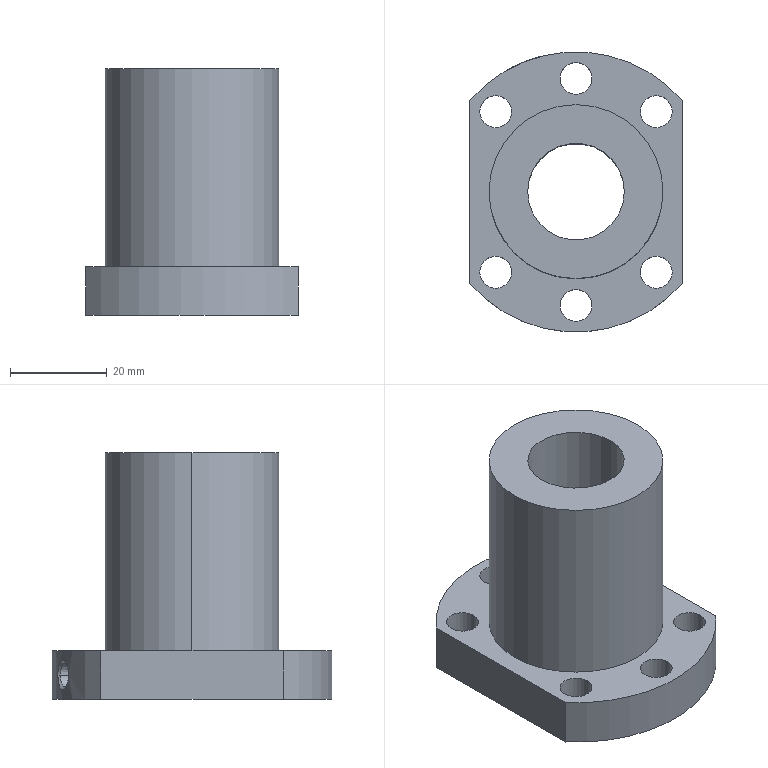Part | SolidWorks | features BaseBody 1 | 1 solid | 32 faces | box 44 x 58 x 51 mm | volume 46253 mm3 | cylinder 22 | plane 6 | cone 4 | commonest cylinder face diameters 6.6 x12 3 x2 4.917 x2 20 x2 36 x2 58 x2
STEP:
#1=CARTESIAN_POINT('',(-10.,0.,-61.));
#2=VERTEX_POINT('',#1);
#3=CARTESIAN_POINT('',(10.,0.,-61.));
#4=VERTEX_POINT('',#3);
#5=CARTESIAN_POINT('',(0.,0.,-61.));
#6=DIRECTION('',(0.,0.,1.));
#7=DIRECTION('',(1.,0.,0.));
#8=AXIS2_PLACEMENT_3D('',#5,#6,#7);
#9=CIRCLE('',#8,10.);
#10=EDGE_CURVE('',#2,#4,#9,.T.);
#11=ORIENTED_EDGE('',*,*,#10,.T.);
#12=CARTESIAN_POINT('',(10.,0.,-112.));
#13=VERTEX_POINT('',#12);
#14=CARTESIAN_POINT('',(10.,0.,-61.));
#15=DIRECTION('',(0.,0.,-1.));
#16=VECTOR('',#15,1000.);
#17=LINE('',#14,#16);
#18=EDGE_CURVE('',#4,#13,#17,.T.);
#19=ORIENTED_EDGE('',*,*,#18,.T.);
#20=CARTESIAN_POINT('',(-10.,0.,-112.));
#21=VERTEX_POINT('',#20);
#22=CARTESIAN_POINT('',(0.,0.,-112.));
#23=DIRECTION('',(0.,0.,1.));
#24=DIRECTION('',(1.,0.,0.));
#25=AXIS2_PLACEMENT_3D('',#22,#23,#24);
#26=CIRCLE('',#25,10.);
#27=EDGE_CURVE('',#21,#13,#26,.T.);
#28=ORIENTED_EDGE('',*,*,#27,.F.);
#29=CARTESIAN_POINT('',(-10.,0.,-61.));
#30=DIRECTION('',(0.,0.,-1.));
#31=VECTOR('',#30,1000.);
#32=LINE('',#29,#31);
#33=EDGE_CURVE('',#2,#21,#32,.T.);
#34=ORIENTED_EDGE('',*,*,#33,.F.);
#35=EDGE_LOOP('',(#11,#19,#28,#34));
#36=FACE_OUTER_BOUND('',#35,.T.);
#37=CARTESIAN_POINT('',(0.,0.,-61.));
#38=DIRECTION('',(0.,0.,-1.));
#39=DIRECTION('',(-1.,0.,0.));
#40=AXIS2_PLACEMENT_3D('',#37,#38,#39);
#41=CYLINDRICAL_SURFACE('',#40,10.);
#42=ADVANCED_FACE('',(#36),#41,.F.);
#43=CARTESIAN_POINT('',(-11.472,21.271,-107.));
#44=VERTEX_POINT('',#43);
#45=CARTESIAN_POINT('',(-6.929,23.152,-107.));
#46=VERTEX_POINT('',#45);
#47=CARTESIAN_POINT('',(-9.2,22.211,-107.));
#48=DIRECTION('',(0.3827,-0.9239,0.));
#49=DIRECTION('',(0.9239,0.3827,0.));
#50=AXIS2_PLACEMENT_3D('',#47,#48,#49);
#51=CIRCLE('',#50,2.459);
#52=EDGE_CURVE('',#44,#46,#51,.T.);
#53=ORIENTED_EDGE('',*,*,#52,.F.);
#54=CARTESIAN_POINT('',(-11.765,20.563,-107.));
#55=VERTEX_POINT('',#54);
#56=CARTESIAN_POINT('',(-11.472,21.271,-107.));
#57=DIRECTION('',(-0.3827,-0.9239,0.));
#58=VECTOR('',#57,1000.);
#59=LINE('',#56,#58);
#60=EDGE_CURVE('',#44,#55,#59,.T.);
#61=ORIENTED_EDGE('',*,*,#60,.T.);
#62=CARTESIAN_POINT('',(-6.221,22.859,-107.));
#63=VERTEX_POINT('',#62);
#64=CARTESIAN_POINT('',(-8.993,21.711,-107.));
#65=DIRECTION('',(0.3827,-0.9239,0.));
#66=DIRECTION('',(0.9239,0.3827,0.));
#67=AXIS2_PLACEMENT_3D('',#64,#65,#66);
#68=CIRCLE('',#67,3.);
#69=EDGE_CURVE('',#55,#63,#68,.T.);
#70=ORIENTED_EDGE('',*,*,#69,.T.);
#71=CARTESIAN_POINT('',(-6.929,23.152,-107.));
#72=DIRECTION('',(0.9239,-0.3827,0.));
#73=VECTOR('',#72,1000.);
#74=LINE('',#71,#73);
#75=EDGE_CURVE('',#46,#63,#74,.T.);
#76=ORIENTED_EDGE('',*,*,#75,.F.);
#77=EDGE_LOOP('',(#53,#61,#70,#76));
#78=FACE_OUTER_BOUND('',#77,.T.);
#79=CARTESIAN_POINT('',(-9.2,22.211,-107.));
#80=DIRECTION('',(0.3827,-0.9239,0.));
#81=DIRECTION('',(0.9239,0.3827,0.));
#82=AXIS2_PLACEMENT_3D('',#79,#80,#81);
#83=CONICAL_SURFACE('',#82,2.459,0.7854);
#84=ADVANCED_FACE('',(#78),#83,.F.);
#85=CARTESIAN_POINT('',(-13.162,25.351,-107.));
#86=VERTEX_POINT('',#85);
#87=CARTESIAN_POINT('',(-8.619,27.233,-107.));
#88=VERTEX_POINT('',#87);
#89=CARTESIAN_POINT('',(-10.891,26.292,-107.));
#90=DIRECTION('',(0.3827,-0.9239,0.));
#91=DIRECTION('',(0.9239,0.3827,0.));
#92=AXIS2_PLACEMENT_3D('',#89,#90,#91);
#93=CIRCLE('',#92,2.459);
#94=EDGE_CURVE('',#86,#88,#93,.T.);
#95=ORIENTED_EDGE('',*,*,#94,.F.);
#96=CARTESIAN_POINT('',(-5.279,6.319,-107.));
#97=DIRECTION('',(0.3827,-0.9239,0.));
#98=VECTOR('',#97,1000.);
#99=LINE('',#96,#98);
#100=EDGE_CURVE('',#86,#44,#99,.T.);
#101=ORIENTED_EDGE('',*,*,#100,.T.);
#102=ORIENTED_EDGE('',*,*,#52,.T.);
#103=CARTESIAN_POINT('',(-0.7358,8.201,-107.));
#104=DIRECTION('',(0.3827,-0.9239,0.));
#105=VECTOR('',#104,1000.);
#106=LINE('',#103,#105);
#107=EDGE_CURVE('',#88,#46,#106,.T.);
#108=ORIENTED_EDGE('',*,*,#107,.F.);
#109=EDGE_LOOP('',(#95,#101,#102,#108));
#110=FACE_OUTER_BOUND('',#109,.T.);
#111=CARTESIAN_POINT('',(-3.007,7.26,-107.));
#112=DIRECTION('',(0.3827,-0.9239,0.));
#113=DIRECTION('',(0.9239,0.3827,0.));
#114=AXIS2_PLACEMENT_3D('',#111,#112,#113);
#115=CYLINDRICAL_SURFACE('',#114,2.459);
#116=ADVANCED_FACE('',(#110),#115,.F.);
#117=ORIENTED_EDGE('',*,*,#94,.T.);
#118=CARTESIAN_POINT('',(-8.403,27.756,-107.));
#119=VERTEX_POINT('',#118);
#120=CARTESIAN_POINT('',(-8.326,27.941,-107.));
#121=DIRECTION('',(0.3827,0.9239,0.));
#122=VECTOR('',#121,1000.);
#123=LINE('',#120,#122);
#124=EDGE_CURVE('',#88,#119,#123,.T.);
#125=ORIENTED_EDGE('',*,*,#124,.T.);
#126=CARTESIAN_POINT('',(-13.685,25.568,-107.));
#127=VERTEX_POINT('',#126);
#128=CARTESIAN_POINT('',(-8.403,27.756,-107.));
#129=CARTESIAN_POINT('',(-8.403,27.756,-107.193));
#130=CARTESIAN_POINT('',(-8.42,27.751,-107.384));
#131=CARTESIAN_POINT('',(-8.486,27.731,-107.759));
#132=CARTESIAN_POINT('',(-8.537,27.715,-107.945));
#133=CARTESIAN_POINT('',(-8.67,27.674,-108.304));
#134=CARTESIAN_POINT('',(-8.751,27.648,-108.475));
#135=CARTESIAN_POINT('',(-8.943,27.587,-108.799));
#136=CARTESIAN_POINT('',(-9.056,27.55,-108.954));
#137=CARTESIAN_POINT('',(-9.304,27.467,-109.234));
#138=CARTESIAN_POINT('',(-9.439,27.421,-109.361));
#139=CARTESIAN_POINT('',(-9.732,27.319,-109.584));
#140=CARTESIAN_POINT('',(-9.891,27.262,-109.682));
#141=CARTESIAN_POINT('',(-10.219,27.141,-109.838));
#142=CARTESIAN_POINT('',(-10.388,27.076,-109.898));
#143=CARTESIAN_POINT('',(-10.739,26.939,-109.979));
#144=CARTESIAN_POINT('',(-10.917,26.867,-110.));
#145=CARTESIAN_POINT('',(-11.27,26.721,-110.));
#146=CARTESIAN_POINT('',(-11.448,26.645,-109.98));
#147=CARTESIAN_POINT('',(-11.793,26.495,-109.9));
#148=CARTESIAN_POINT('',(-11.959,26.42,-109.841));
#149=CARTESIAN_POINT('',(-12.277,26.274,-109.685));
#150=CARTESIAN_POINT('',(-12.43,26.201,-109.588));
#151=CARTESIAN_POINT('',(-12.71,26.067,-109.365));
#152=CARTESIAN_POINT('',(-12.84,26.003,-109.239));
#153=CARTESIAN_POINT('',(-13.076,25.885,-108.956));
#154=CARTESIAN_POINT('',(-13.18,25.832,-108.804));
#155=CARTESIAN_POINT('',(-13.36,25.739,-108.48));
#156=CARTESIAN_POINT('',(-13.437,25.699,-108.306));
#157=CARTESIAN_POINT('',(-13.56,25.634,-107.948));
#158=CARTESIAN_POINT('',(-13.607,25.61,-107.764));
#159=CARTESIAN_POINT('',(-13.669,25.577,-107.387));
#160=CARTESIAN_POINT('',(-13.685,25.568,-107.194));
#161=CARTESIAN_POINT('',(-13.685,25.568,-107.));
#162=B_SPLINE_CURVE_WITH_KNOTS('',3,(#128,#129,#130,#131,#132,#133,#134,#135,#136,#137,#138,#139,#140,#141,#142,#143,#144,#145,#146,#147,#148,#149,#150,#151,#152,#153,#154,#155,#156,#157,#158,#159,#160,#161),.UNSPECIFIED.,.F.,.F.,(4,2,2,2,2,2,2,2,2,2,2,2,2,2,2,2,4),(0.000000001,0.0005722,0.001144,0.001717,0.002289,0.002861,0.003433,0.004006,0.004578,0.00515,0.005722,0.006295,0.006867,0.007439,0.008011,0.008584,0.009156),.UNSPECIFIED.);
#163=EDGE_CURVE('',#119,#127,#162,.T.);
#164=ORIENTED_EDGE('',*,*,#163,.T.);
#165=CARTESIAN_POINT('',(-13.869,25.644,-107.));
#166=DIRECTION('',(-0.9239,0.3827,0.));
#167=VECTOR('',#166,1000.);
#168=LINE('',#165,#167);
#169=EDGE_CURVE('',#86,#127,#168,.T.);
#170=ORIENTED_EDGE('',*,*,#169,.F.);
#171=EDGE_LOOP('',(#117,#125,#164,#170));
#172=FACE_OUTER_BOUND('',#171,.T.);
#173=CARTESIAN_POINT('',(-11.098,26.793,-107.));
#174=DIRECTION('',(-0.3827,0.9239,0.));
#175=DIRECTION('',(-0.9239,-0.3827,0.));
#176=AXIS2_PLACEMENT_3D('',#173,#174,#175);
#177=CONICAL_SURFACE('',#176,3.,0.7854);
#178=ADVANCED_FACE('',(#172),#177,.F.);
#179=CARTESIAN_POINT('',(-19.917,16.617,-102.));
#180=VERTEX_POINT('',#179);
#181=CARTESIAN_POINT('',(-13.317,16.617,-102.));
#182=VERTEX_POINT('',#181);
#183=CARTESIAN_POINT('',(-16.617,16.617,-102.));
#184=DIRECTION('',(0.,0.,1.));
#185=DIRECTION('',(1.,0.,0.));
#186=AXIS2_PLACEMENT_3D('',#183,#184,#185);
#187=CIRCLE('',#186,3.3);
#188=EDGE_CURVE('',#180,#182,#187,.T.);
#189=ORIENTED_EDGE('',*,*,#188,.T.);
#190=CARTESIAN_POINT('',(-13.317,16.617,-112.));
#191=VERTEX_POINT('',#190);
#192=CARTESIAN_POINT('',(-13.317,16.617,-102.));
#193=DIRECTION('',(0.,0.,-1.));
#194=VECTOR('',#193,1000.);
#195=LINE('',#192,#194);
#196=EDGE_CURVE('',#182,#191,#195,.T.);
#197=ORIENTED_EDGE('',*,*,#196,.T.);
#198=CARTESIAN_POINT('',(-19.917,16.617,-112.));
#199=VERTEX_POINT('',#198);
#200=CARTESIAN_POINT('',(-16.617,16.617,-112.));
#201=DIRECTION('',(0.,0.,1.));
#202=DIRECTION('',(1.,0.,0.));
#203=AXIS2_PLACEMENT_3D('',#200,#201,#202);
#204=CIRCLE('',#203,3.3);
#205=EDGE_CURVE('',#199,#191,#204,.T.);
#206=ORIENTED_EDGE('',*,*,#205,.F.);
#207=CARTESIAN_POINT('',(-19.917,16.617,-102.));
#208=DIRECTION('',(0.,0.,-1.));
#209=VECTOR('',#208,1000.);
#210=LINE('',#207,#209);
#211=EDGE_CURVE('',#180,#199,#210,.T.);
#212=ORIENTED_EDGE('',*,*,#211,.F.);
#213=EDGE_LOOP('',(#189,#197,#206,#212));
#214=FACE_OUTER_BOUND('',#213,.T.);
#215=CARTESIAN_POINT('',(-16.617,16.617,-102.));
#216=DIRECTION('',(0.,0.,-1.));
#217=DIRECTION('',(-1.,0.,0.));
#218=AXIS2_PLACEMENT_3D('',#215,#216,#217);
#219=CYLINDRICAL_SURFACE('',#218,3.3);
#220=ADVANCED_FACE('',(#214),#219,.F.);
#221=CARTESIAN_POINT('',(-19.917,-16.617,-102.));
#222=VERTEX_POINT('',#221);
#223=CARTESIAN_POINT('',(-13.317,-16.617,-102.));
#224=VERTEX_POINT('',#223);
#225=CARTESIAN_POINT('',(-16.617,-16.617,-102.));
#226=DIRECTION('',(0.,0.,1.));
#227=DIRECTION('',(1.,0.,0.));
#228=AXIS2_PLACEMENT_3D('',#225,#226,#227);
#229=CIRCLE('',#228,3.3);
#230=EDGE_CURVE('',#222,#224,#229,.T.);
#231=ORIENTED_EDGE('',*,*,#230,.T.);
#232=CARTESIAN_POINT('',(-13.317,-16.617,-112.));
#233=VERTEX_POINT('',#232);
#234=CARTESIAN_POINT('',(-13.317,-16.617,-102.));
#235=DIRECTION('',(0.,0.,-1.));
#236=VECTOR('',#235,1000.);
#237=LINE('',#234,#236);
#238=EDGE_CURVE('',#224,#233,#237,.T.);
#239=ORIENTED_EDGE('',*,*,#238,.T.);
#240=CARTESIAN_POINT('',(-19.917,-16.617,-112.));
#241=VERTEX_POINT('',#240);
#242=CARTESIAN_POINT('',(-16.617,-16.617,-112.));
#243=DIRECTION('',(0.,0.,1.));
#244=DIRECTION('',(1.,0.,0.));
#245=AXIS2_PLACEMENT_3D('',#242,#243,#244);
#246=CIRCLE('',#245,3.3);
#247=EDGE_CURVE('',#241,#233,#246,.T.);
#248=ORIENTED_EDGE('',*,*,#247,.F.);
#249=CARTESIAN_POINT('',(-19.917,-16.617,-102.));
#250=DIRECTION('',(0.,0.,-1.));
#251=VECTOR('',#250,1000.);
#252=LINE('',#249,#251);
#253=EDGE_CURVE('',#222,#241,#252,.T.);
#254=ORIENTED_EDGE('',*,*,#253,.F.);
#255=EDGE_LOOP('',(#231,#239,#248,#254));
#256=FACE_OUTER_BOUND('',#255,.T.);
#257=CARTESIAN_POINT('',(-16.617,-16.617,-102.));
#258=DIRECTION('',(0.,0.,-1.));
#259=DIRECTION('',(-1.,0.,0.));
#260=AXIS2_PLACEMENT_3D('',#257,#258,#259);
#261=CYLINDRICAL_SURFACE('',#260,3.3);
#262=ADVANCED_FACE('',(#256),#261,.F.);
#263=CARTESIAN_POINT('',(-3.3,-23.5,-102.));
#264=VERTEX_POINT('',#263);
#265=CARTESIAN_POINT('',(3.3,-23.5,-102.));
#266=VERTEX_POINT('',#265);
#267=CARTESIAN_POINT('',(0.,-23.5,-102.));
#268=DIRECTION('',(0.,0.,1.));
#269=DIRECTION('',(1.,0.,0.));
#270=AXIS2_PLACEMENT_3D('',#267,#268,#269);
#271=CIRCLE('',#270,3.3);
#272=EDGE_CURVE('',#264,#266,#271,.T.);
#273=ORIENTED_EDGE('',*,*,#272,.T.);
#274=CARTESIAN_POINT('',(3.3,-23.5,-112.));
#275=VERTEX_POINT('',#274);
#276=CARTESIAN_POINT('',(3.3,-23.5,-102.));
#277=DIRECTION('',(0.,0.,-1.));
#278=VECTOR('',#277,1000.);
#279=LINE('',#276,#278);
#280=EDGE_CURVE('',#266,#275,#279,.T.);
#281=ORIENTED_EDGE('',*,*,#280,.T.);
#282=CARTESIAN_POINT('',(-3.3,-23.5,-112.));
#283=VERTEX_POINT('',#282);
#284=CARTESIAN_POINT('',(0.,-23.5,-112.));
#285=DIRECTION('',(0.,0.,1.));
#286=DIRECTION('',(1.,0.,0.));
#287=AXIS2_PLACEMENT_3D('',#284,#285,#286);
#288=CIRCLE('',#287,3.3);
#289=EDGE_CURVE('',#283,#275,#288,.T.);
#290=ORIENTED_EDGE('',*,*,#289,.F.);
#291=CARTESIAN_POINT('',(-3.3,-23.5,-102.));
#292=DIRECTION('',(0.,0.,-1.));
#293=VECTOR('',#292,1000.);
#294=LINE('',#291,#293);
#295=EDGE_CURVE('',#264,#283,#294,.T.);
#296=ORIENTED_EDGE('',*,*,#295,.F.);
#297=EDGE_LOOP('',(#273,#281,#290,#296));
#298=FACE_OUTER_BOUND('',#297,.T.);
#299=CARTESIAN_POINT('',(0.,-23.5,-102.));
#300=DIRECTION('',(0.,0.,-1.));
#301=DIRECTION('',(-1.,0.,0.));
#302=AXIS2_PLACEMENT_3D('',#299,#300,#301);
#303=CYLINDRICAL_SURFACE('',#302,3.3);
#304=ADVANCED_FACE('',(#298),#303,.F.);
#305=CARTESIAN_POINT('',(-3.3,23.5,-102.));
#306=VERTEX_POINT('',#305);
#307=CARTESIAN_POINT('',(3.3,23.5,-102.));
#308=VERTEX_POINT('',#307);
#309=CARTESIAN_POINT('',(0.,23.5,-102.));
#310=DIRECTION('',(0.,0.,1.));
#311=DIRECTION('',(1.,0.,0.));
#312=AXIS2_PLACEMENT_3D('',#309,#310,#311);
#313=CIRCLE('',#312,3.3);
#314=EDGE_CURVE('',#306,#308,#313,.T.);
#315=ORIENTED_EDGE('',*,*,#314,.T.);
#316=CARTESIAN_POINT('',(3.3,23.5,-112.));
#317=VERTEX_POINT('',#316);
#318=CARTESIAN_POINT('',(3.3,23.5,-102.));
#319=DIRECTION('',(0.,0.,-1.));
#320=VECTOR('',#319,1000.);
#321=LINE('',#318,#320);
#322=EDGE_CURVE('',#308,#317,#321,.T.);
#323=ORIENTED_EDGE('',*,*,#322,.T.);
#324=CARTESIAN_POINT('',(-3.3,23.5,-112.));
#325=VERTEX_POINT('',#324);
#326=CARTESIAN_POINT('',(0.,23.5,-112.));
#327=DIRECTION('',(0.,0.,1.));
#328=DIRECTION('',(1.,0.,0.));
#329=AXIS2_PLACEMENT_3D('',#326,#327,#328);
#330=CIRCLE('',#329,3.3);
#331=EDGE_CURVE('',#325,#317,#330,.T.);
#332=ORIENTED_EDGE('',*,*,#331,.F.);
#333=CARTESIAN_POINT('',(-3.3,23.5,-102.));
#334=DIRECTION('',(0.,0.,-1.));
#335=VECTOR('',#334,1000.);
#336=LINE('',#333,#335);
#337=EDGE_CURVE('',#306,#325,#336,.T.);
#338=ORIENTED_EDGE('',*,*,#337,.F.);
#339=EDGE_LOOP('',(#315,#323,#332,#338));
#340=FACE_OUTER_BOUND('',#339,.T.);
#341=CARTESIAN_POINT('',(0.,23.5,-102.));
#342=DIRECTION('',(0.,0.,-1.));
#343=DIRECTION('',(-1.,0.,0.));
#344=AXIS2_PLACEMENT_3D('',#341,#342,#343);
#345=CYLINDRICAL_SURFACE('',#344,3.3);
#346=ADVANCED_FACE('',(#340),#345,.F.);
#347=CARTESIAN_POINT('',(13.317,-16.617,-102.));
#348=VERTEX_POINT('',#347);
#349=CARTESIAN_POINT('',(19.917,-16.617,-102.));
#350=VERTEX_POINT('',#349);
#351=CARTESIAN_POINT('',(16.617,-16.617,-102.));
#352=DIRECTION('',(0.,0.,1.));
#353=DIRECTION('',(1.,0.,0.));
#354=AXIS2_PLACEMENT_3D('',#351,#352,#353);
#355=CIRCLE('',#354,3.3);
#356=EDGE_CURVE('',#348,#350,#355,.T.);
#357=ORIENTED_EDGE('',*,*,#356,.T.);
#358=CARTESIAN_POINT('',(19.917,-16.617,-112.));
#359=VERTEX_POINT('',#358);
#360=CARTESIAN_POINT('',(19.917,-16.617,-102.));
#361=DIRECTION('',(0.,0.,-1.));
#362=VECTOR('',#361,1000.);
#363=LINE('',#360,#362);
#364=EDGE_CURVE('',#350,#359,#363,.T.);
#365=ORIENTED_EDGE('',*,*,#364,.T.);
#366=CARTESIAN_POINT('',(13.317,-16.617,-112.));
#367=VERTEX_POINT('',#366);
#368=CARTESIAN_POINT('',(16.617,-16.617,-112.));
#369=DIRECTION('',(0.,0.,1.));
#370=DIRECTION('',(1.,0.,0.));
#371=AXIS2_PLACEMENT_3D('',#368,#369,#370);
#372=CIRCLE('',#371,3.3);
#373=EDGE_CURVE('',#367,#359,#372,.T.);
#374=ORIENTED_EDGE('',*,*,#373,.F.);
#375=CARTESIAN_POINT('',(13.317,-16.617,-102.));
#376=DIRECTION('',(0.,0.,-1.));
#377=VECTOR('',#376,1000.);
#378=LINE('',#375,#377);
#379=EDGE_CURVE('',#348,#367,#378,.T.);
#380=ORIENTED_EDGE('',*,*,#379,.F.);
#381=EDGE_LOOP('',(#357,#365,#374,#380));
#382=FACE_OUTER_BOUND('',#381,.T.);
#383=CARTESIAN_POINT('',(16.617,-16.617,-102.));
#384=DIRECTION('',(0.,0.,-1.));
#385=DIRECTION('',(-1.,0.,0.));
#386=AXIS2_PLACEMENT_3D('',#383,#384,#385);
#387=CYLINDRICAL_SURFACE('',#386,3.3);
#388=ADVANCED_FACE('',(#382),#387,.F.);
#389=CARTESIAN_POINT('',(13.317,16.617,-102.));
#390=VERTEX_POINT('',#389);
#391=CARTESIAN_POINT('',(19.917,16.617,-102.));
#392=VERTEX_POINT('',#391);
#393=CARTESIAN_POINT('',(16.617,16.617,-102.));
#394=DIRECTION('',(0.,0.,1.));
#395=DIRECTION('',(1.,0.,0.));
#396=AXIS2_PLACEMENT_3D('',#393,#394,#395);
#397=CIRCLE('',#396,3.3);
#398=EDGE_CURVE('',#390,#392,#397,.T.);
#399=ORIENTED_EDGE('',*,*,#398,.T.);
#400=CARTESIAN_POINT('',(19.917,16.617,-112.));
#401=VERTEX_POINT('',#400);
#402=CARTESIAN_POINT('',(19.917,16.617,-102.));
#403=DIRECTION('',(0.,0.,-1.));
#404=VECTOR('',#403,1000.);
#405=LINE('',#402,#404);
#406=EDGE_CURVE('',#392,#401,#405,.T.);
#407=ORIENTED_EDGE('',*,*,#406,.T.);
#408=CARTESIAN_POINT('',(13.317,16.617,-112.));
#409=VERTEX_POINT('',#408);
#410=CARTESIAN_POINT('',(16.617,16.617,-112.));
#411=DIRECTION('',(0.,0.,1.));
#412=DIRECTION('',(1.,0.,0.));
#413=AXIS2_PLACEMENT_3D('',#410,#411,#412);
#414=CIRCLE('',#413,3.3);
#415=EDGE_CURVE('',#409,#401,#414,.T.);
#416=ORIENTED_EDGE('',*,*,#415,.F.);
#417=CARTESIAN_POINT('',(13.317,16.617,-102.));
#418=DIRECTION('',(0.,0.,-1.));
#419=VECTOR('',#418,1000.);
#420=LINE('',#417,#419);
#421=EDGE_CURVE('',#390,#409,#420,.T.);
#422=ORIENTED_EDGE('',*,*,#421,.F.);
#423=EDGE_LOOP('',(#399,#407,#416,#422));
#424=FACE_OUTER_BOUND('',#423,.T.);
#425=CARTESIAN_POINT('',(16.617,16.617,-102.));
#426=DIRECTION('',(0.,0.,-1.));
#427=DIRECTION('',(-1.,0.,0.));
#428=AXIS2_PLACEMENT_3D('',#425,#426,#427);
#429=CYLINDRICAL_SURFACE('',#428,3.3);
#430=ADVANCED_FACE('',(#424),#429,.F.);
#431=CARTESIAN_POINT('',(18.,0.,-61.));
#432=VERTEX_POINT('',#431);
#433=CARTESIAN_POINT('',(-18.,0.,-61.));
#434=VERTEX_POINT('',#433);
#435=CARTESIAN_POINT('',(0.,0.,-61.));
#436=DIRECTION('',(0.,0.,1.));
#437=DIRECTION('',(1.,0.,0.));
#438=AXIS2_PLACEMENT_3D('',#435,#436,#437);
#439=CIRCLE('',#438,18.);
#440=EDGE_CURVE('',#432,#434,#439,.T.);
#441=ORIENTED_EDGE('',*,*,#440,.F.);
#442=CARTESIAN_POINT('',(18.,0.,-102.));
#443=VERTEX_POINT('',#442);
#444=CARTESIAN_POINT('',(18.,0.,-61.));
#445=DIRECTION('',(0.,0.,-1.));
#446=VECTOR('',#445,1000.);
#447=LINE('',#444,#446);
#448=EDGE_CURVE('',#432,#443,#447,.T.);
#449=ORIENTED_EDGE('',*,*,#448,.T.);
#450=CARTESIAN_POINT('',(-18.,0.,-102.));
#451=VERTEX_POINT('',#450);
#452=CARTESIAN_POINT('',(0.,0.,-102.));
#453=DIRECTION('',(0.,0.,1.));
#454=DIRECTION('',(1.,0.,0.));
#455=AXIS2_PLACEMENT_3D('',#452,#453,#454);
#456=CIRCLE('',#455,18.);
#457=EDGE_CURVE('',#443,#451,#456,.T.);
#458=ORIENTED_EDGE('',*,*,#457,.T.);
#459=CARTESIAN_POINT('',(-18.,0.,-61.));
#460=DIRECTION('',(0.,0.,-1.));
#461=VECTOR('',#460,1000.);
#462=LINE('',#459,#461);
#463=EDGE_CURVE('',#434,#451,#462,.T.);
#464=ORIENTED_EDGE('',*,*,#463,.F.);
#465=EDGE_LOOP('',(#441,#449,#458,#464));
#466=FACE_OUTER_BOUND('',#465,.T.);
#467=CARTESIAN_POINT('',(0.,0.,-61.));
#468=DIRECTION('',(0.,0.,-1.));
#469=DIRECTION('',(-1.,0.,0.));
#470=AXIS2_PLACEMENT_3D('',#467,#468,#469);
#471=CYLINDRICAL_SURFACE('',#470,18.);
#472=ADVANCED_FACE('',(#466),#471,.T.);
#473=CARTESIAN_POINT('',(-10.379,21.137,-107.));
#474=VERTEX_POINT('',#473);
#475=CARTESIAN_POINT('',(-7.607,22.285,-107.));
#476=VERTEX_POINT('',#475);
#477=CARTESIAN_POINT('',(-8.993,21.711,-107.));
#478=DIRECTION('',(0.3827,-0.9239,0.));
#479=DIRECTION('',(0.9239,0.3827,0.));
#480=AXIS2_PLACEMENT_3D('',#477,#478,#479);
#481=CIRCLE('',#480,1.5);
#482=EDGE_CURVE('',#474,#476,#481,.T.);
#483=ORIENTED_EDGE('',*,*,#482,.F.);
#484=CARTESIAN_POINT('',(-5.169,8.56,-107.));
#485=VERTEX_POINT('',#484);
#486=CARTESIAN_POINT('',(-4.393,6.686,-107.));
#487=DIRECTION('',(0.3827,-0.9239,0.));
#488=VECTOR('',#487,1000.);
#489=LINE('',#486,#488);
#490=EDGE_CURVE('',#474,#485,#489,.T.);
#491=ORIENTED_EDGE('',*,*,#490,.T.);
#492=CARTESIAN_POINT('',(-2.398,9.708,-107.));
#493=VERTEX_POINT('',#492);
#494=CARTESIAN_POINT('',(-5.169,8.56,-107.));
#495=CARTESIAN_POINT('',(-5.169,8.56,-107.099));
#496=CARTESIAN_POINT('',(-5.161,8.565,-107.197));
#497=CARTESIAN_POINT('',(-5.128,8.585,-107.389));
#498=CARTESIAN_POINT('',(-5.103,8.6,-107.484));
#499=CARTESIAN_POINT('',(-5.037,8.639,-107.666));
#500=CARTESIAN_POINT('',(-4.997,8.662,-107.752));
#501=CARTESIAN_POINT('',(-4.902,8.716,-107.915));
#502=CARTESIAN_POINT('',(-4.846,8.748,-107.992));
#503=CARTESIAN_POINT('',(-4.663,8.847,-108.199));
#504=CARTESIAN_POINT('',(-4.514,8.925,-108.311));
#505=CARTESIAN_POINT('',(-4.189,9.082,-108.46));
#506=CARTESIAN_POINT('',(-4.009,9.163,-108.5));
#507=CARTESIAN_POINT('',(-3.737,9.276,-108.5));
#508=CARTESIAN_POINT('',(-3.645,9.313,-108.49));
#509=CARTESIAN_POINT('',(-3.465,9.381,-108.452));
#510=CARTESIAN_POINT('',(-3.377,9.413,-108.424));
#511=CARTESIAN_POINT('',(-3.119,9.503,-108.311));
#512=CARTESIAN_POINT('',(-2.961,9.553,-108.201));
#513=CARTESIAN_POINT('',(-2.758,9.612,-107.991));
#514=CARTESIAN_POINT('',(-2.698,9.629,-107.916));
#515=CARTESIAN_POINT('',(-2.593,9.658,-107.754));
#516=CARTESIAN_POINT('',(-2.547,9.67,-107.666));
#517=CARTESIAN_POINT('',(-2.436,9.699,-107.394));
#518=CARTESIAN_POINT('',(-2.398,9.708,-107.198));
#519=CARTESIAN_POINT('',(-2.398,9.708,-107.));
#520=B_SPLINE_CURVE_WITH_KNOTS('',3,(#494,#495,#496,#497,#498,#499,#500,#501,#502,#503,#504,#505,#506,#507,#508,#509,#510,#511,#512,#513,#514,#515,#516,#517,#518,#519),.UNSPECIFIED.,.F.,.F.,(4,2,2,2,2,2,2,2,2,2,2,2,4),(0.,0.0002934,0.0005869,0.0008803,0.001174,0.001761,0.002348,0.002641,0.002934,0.003521,0.003815,0.004108,0.004695),.UNSPECIFIED.);
#521=EDGE_CURVE('',#485,#493,#520,.T.);
#522=ORIENTED_EDGE('',*,*,#521,.T.);
#523=CARTESIAN_POINT('',(-1.621,7.834,-107.));
#524=DIRECTION('',(0.3827,-0.9239,0.));
#525=VECTOR('',#524,1000.);
#526=LINE('',#523,#525);
#527=EDGE_CURVE('',#476,#493,#526,.T.);
#528=ORIENTED_EDGE('',*,*,#527,.F.);
#529=EDGE_LOOP('',(#483,#491,#522,#528));
#530=FACE_OUTER_BOUND('',#529,.T.);
#531=CARTESIAN_POINT('',(-3.007,7.26,-107.));
#532=DIRECTION('',(0.3827,-0.9239,0.));
#533=DIRECTION('',(0.9239,0.3827,0.));
#534=AXIS2_PLACEMENT_3D('',#531,#532,#533);
#535=CYLINDRICAL_SURFACE('',#534,1.5);
#536=ADVANCED_FACE('',(#530),#535,.F.);
#537=CARTESIAN_POINT('',(-8.993,21.711,-107.));
#538=DIRECTION('',(0.3827,-0.9239,0.));
#539=DIRECTION('',(0.9239,0.3827,0.));
#540=AXIS2_PLACEMENT_3D('',#537,#538,#539);
#541=CIRCLE('',#540,1.5);
#542=EDGE_CURVE('',#476,#474,#541,.T.);
#543=ORIENTED_EDGE('',*,*,#542,.T.);
#544=ORIENTED_EDGE('',*,*,#482,.T.);
#545=EDGE_LOOP('',(#543,#544));
#546=FACE_BOUND('',#545,.T.);
#547=CARTESIAN_POINT('',(-8.993,21.711,-107.));
#548=DIRECTION('',(0.3827,-0.9239,0.));
#549=DIRECTION('',(0.9239,0.3827,0.));
#550=AXIS2_PLACEMENT_3D('',#547,#548,#549);
#551=CIRCLE('',#550,3.);
#552=EDGE_CURVE('',#63,#55,#551,.T.);
#553=ORIENTED_EDGE('',*,*,#552,.F.);
#554=ORIENTED_EDGE('',*,*,#69,.F.);
#555=EDGE_LOOP('',(#553,#554));
#556=FACE_OUTER_BOUND('',#555,.T.);
#557=CARTESIAN_POINT('',(-6.221,22.859,-107.));
#558=DIRECTION('',(-0.3827,0.9239,0.));
#559=DIRECTION('',(0.,0.,1.));
#560=AXIS2_PLACEMENT_3D('',#557,#558,#559);
#561=PLANE('',#560);
#562=ADVANCED_FACE('',(#546,#556),#561,.T.);
#563=ORIENTED_EDGE('',*,*,#415,.T.);
#564=CARTESIAN_POINT('',(16.617,16.617,-112.));
#565=DIRECTION('',(0.,0.,1.));
#566=DIRECTION('',(1.,0.,0.));
#567=AXIS2_PLACEMENT_3D('',#564,#565,#566);
#568=CIRCLE('',#567,3.3);
#569=EDGE_CURVE('',#401,#409,#568,.T.);
#570=ORIENTED_EDGE('',*,*,#569,.T.);
#571=EDGE_LOOP('',(#563,#570));
#572=FACE_BOUND('',#571,.T.);
#573=ORIENTED_EDGE('',*,*,#373,.T.);
#574=CARTESIAN_POINT('',(16.617,-16.617,-112.));
#575=DIRECTION('',(0.,0.,1.));
#576=DIRECTION('',(1.,0.,0.));
#577=AXIS2_PLACEMENT_3D('',#574,#575,#576);
#578=CIRCLE('',#577,3.3);
#579=EDGE_CURVE('',#359,#367,#578,.T.);
#580=ORIENTED_EDGE('',*,*,#579,.T.);
#581=EDGE_LOOP('',(#573,#580));
#582=FACE_BOUND('',#581,.T.);
#583=ORIENTED_EDGE('',*,*,#331,.T.);
#584=CARTESIAN_POINT('',(0.,23.5,-112.));
#585=DIRECTION('',(0.,0.,1.));
#586=DIRECTION('',(1.,0.,0.));
#587=AXIS2_PLACEMENT_3D('',#584,#585,#586);
#588=CIRCLE('',#587,3.3);
#589=EDGE_CURVE('',#317,#325,#588,.T.);
#590=ORIENTED_EDGE('',*,*,#589,.T.);
#591=EDGE_LOOP('',(#583,#590));
#592=FACE_BOUND('',#591,.T.);
#593=ORIENTED_EDGE('',*,*,#289,.T.);
#594=CARTESIAN_POINT('',(0.,-23.5,-112.));
#595=DIRECTION('',(0.,0.,1.));
#596=DIRECTION('',(1.,0.,0.));
#597=AXIS2_PLACEMENT_3D('',#594,#595,#596);
#598=CIRCLE('',#597,3.3);
#599=EDGE_CURVE('',#275,#283,#598,.T.);
#600=ORIENTED_EDGE('',*,*,#599,.T.);
#601=EDGE_LOOP('',(#593,#600));
#602=FACE_BOUND('',#601,.T.);
#603=ORIENTED_EDGE('',*,*,#247,.T.);
#604=CARTESIAN_POINT('',(-16.617,-16.617,-112.));
#605=DIRECTION('',(0.,0.,1.));
#606=DIRECTION('',(1.,0.,0.));
#607=AXIS2_PLACEMENT_3D('',#604,#605,#606);
#608=CIRCLE('',#607,3.3);
#609=EDGE_CURVE('',#233,#241,#608,.T.);
#610=ORIENTED_EDGE('',*,*,#609,.T.);
#611=EDGE_LOOP('',(#603,#610));
#612=FACE_BOUND('',#611,.T.);
#613=ORIENTED_EDGE('',*,*,#205,.T.);
#614=CARTESIAN_POINT('',(-16.617,16.617,-112.));
#615=DIRECTION('',(0.,0.,1.));
#616=DIRECTION('',(1.,0.,0.));
#617=AXIS2_PLACEMENT_3D('',#614,#615,#616);
#618=CIRCLE('',#617,3.3);
#619=EDGE_CURVE('',#191,#199,#618,.T.);
#620=ORIENTED_EDGE('',*,*,#619,.T.);
#621=EDGE_LOOP('',(#613,#620));
#622=FACE_BOUND('',#621,.T.);
#623=ORIENTED_EDGE('',*,*,#27,.T.);
#624=CARTESIAN_POINT('',(0.,0.,-112.));
#625=DIRECTION('',(0.,0.,1.));
#626=DIRECTION('',(1.,0.,0.));
#627=AXIS2_PLACEMENT_3D('',#624,#625,#626);
#628=CIRCLE('',#627,10.);
#629=EDGE_CURVE('',#13,#21,#628,.T.);
#630=ORIENTED_EDGE('',*,*,#629,.T.);
#631=EDGE_LOOP('',(#623,#630));
#632=FACE_BOUND('',#631,.T.);
#633=CARTESIAN_POINT('',(22.,18.894,-112.));
#634=VERTEX_POINT('',#633);
#635=CARTESIAN_POINT('',(-22.,18.894,-112.));
#636=VERTEX_POINT('',#635);
#637=CARTESIAN_POINT('',(0.,0.,-112.));
#638=DIRECTION('',(0.,0.,1.));
#639=DIRECTION('',(1.,0.,0.));
#640=AXIS2_PLACEMENT_3D('',#637,#638,#639);
#641=CIRCLE('',#640,29.);
#642=EDGE_CURVE('',#634,#636,#641,.T.);
#643=ORIENTED_EDGE('',*,*,#642,.F.);
#644=CARTESIAN_POINT('',(22.,-18.894,-112.));
#645=VERTEX_POINT('',#644);
#646=CARTESIAN_POINT('',(22.,-18.894,-112.));
#647=DIRECTION('',(0.,1.,0.));
#648=VECTOR('',#647,1000.);
#649=LINE('',#646,#648);
#650=EDGE_CURVE('',#645,#634,#649,.T.);
#651=ORIENTED_EDGE('',*,*,#650,.F.);
#652=CARTESIAN_POINT('',(-22.,-18.894,-112.));
#653=VERTEX_POINT('',#652);
#654=CARTESIAN_POINT('',(0.,0.,-112.));
#655=DIRECTION('',(0.,0.,1.));
#656=DIRECTION('',(1.,0.,0.));
#657=AXIS2_PLACEMENT_3D('',#654,#655,#656);
#658=CIRCLE('',#657,29.);
#659=EDGE_CURVE('',#653,#645,#658,.T.);
#660=ORIENTED_EDGE('',*,*,#659,.F.);
#661=CARTESIAN_POINT('',(-22.,18.894,-112.));
#662=DIRECTION('',(0.,-1.,0.));
#663=VECTOR('',#662,1000.);
#664=LINE('',#661,#663);
#665=EDGE_CURVE('',#636,#653,#664,.T.);
#666=ORIENTED_EDGE('',*,*,#665,.F.);
#667=EDGE_LOOP('',(#643,#651,#660,#666));
#668=FACE_OUTER_BOUND('',#667,.T.);
#669=CARTESIAN_POINT('',(0.,0.,-112.));
#670=DIRECTION('',(0.,0.,1.));
#671=DIRECTION('',(1.,0.,0.));
#672=AXIS2_PLACEMENT_3D('',#669,#670,#671);
#673=PLANE('',#672);
#674=ADVANCED_FACE('',(#572,#582,#592,#602,#612,#622,#632,#668),#673,.F.);
#675=ORIENTED_EDGE('',*,*,#398,.F.);
#676=CARTESIAN_POINT('',(16.617,16.617,-102.));
#677=DIRECTION('',(0.,0.,1.));
#678=DIRECTION('',(1.,0.,0.));
#679=AXIS2_PLACEMENT_3D('',#676,#677,#678);
#680=CIRCLE('',#679,3.3);
#681=EDGE_CURVE('',#392,#390,#680,.T.);
#682=ORIENTED_EDGE('',*,*,#681,.F.);
#683=EDGE_LOOP('',(#675,#682));
#684=FACE_BOUND('',#683,.T.);
#685=ORIENTED_EDGE('',*,*,#356,.F.);
#686=CARTESIAN_POINT('',(16.617,-16.617,-102.));
#687=DIRECTION('',(0.,0.,1.));
#688=DIRECTION('',(1.,0.,0.));
#689=AXIS2_PLACEMENT_3D('',#686,#687,#688);
#690=CIRCLE('',#689,3.3);
#691=EDGE_CURVE('',#350,#348,#690,.T.);
#692=ORIENTED_EDGE('',*,*,#691,.F.);
#693=EDGE_LOOP('',(#685,#692));
#694=FACE_BOUND('',#693,.T.);
#695=ORIENTED_EDGE('',*,*,#314,.F.);
#696=CARTESIAN_POINT('',(0.,23.5,-102.));
#697=DIRECTION('',(0.,0.,1.));
#698=DIRECTION('',(1.,0.,0.));
#699=AXIS2_PLACEMENT_3D('',#696,#697,#698);
#700=CIRCLE('',#699,3.3);
#701=EDGE_CURVE('',#308,#306,#700,.T.);
#702=ORIENTED_EDGE('',*,*,#701,.F.);
#703=EDGE_LOOP('',(#695,#702));
#704=FACE_BOUND('',#703,.T.);
#705=ORIENTED_EDGE('',*,*,#272,.F.);
#706=CARTESIAN_POINT('',(0.,-23.5,-102.));
#707=DIRECTION('',(0.,0.,1.));
#708=DIRECTION('',(1.,0.,0.));
#709=AXIS2_PLACEMENT_3D('',#706,#707,#708);
#710=CIRCLE('',#709,3.3);
#711=EDGE_CURVE('',#266,#264,#710,.T.);
#712=ORIENTED_EDGE('',*,*,#711,.F.);
#713=EDGE_LOOP('',(#705,#712));
#714=FACE_BOUND('',#713,.T.);
#715=ORIENTED_EDGE('',*,*,#230,.F.);
#716=CARTESIAN_POINT('',(-16.617,-16.617,-102.));
#717=DIRECTION('',(0.,0.,1.));
#718=DIRECTION('',(1.,0.,0.));
#719=AXIS2_PLACEMENT_3D('',#716,#717,#718);
#720=CIRCLE('',#719,3.3);
#721=EDGE_CURVE('',#224,#222,#720,.T.);
#722=ORIENTED_EDGE('',*,*,#721,.F.);
#723=EDGE_LOOP('',(#715,#722));
#724=FACE_BOUND('',#723,.T.);
#725=ORIENTED_EDGE('',*,*,#188,.F.);
#726=CARTESIAN_POINT('',(-16.617,16.617,-102.));
#727=DIRECTION('',(0.,0.,1.));
#728=DIRECTION('',(1.,0.,0.));
#729=AXIS2_PLACEMENT_3D('',#726,#727,#728);
#730=CIRCLE('',#729,3.3);
#731=EDGE_CURVE('',#182,#180,#730,.T.);
#732=ORIENTED_EDGE('',*,*,#731,.F.);
#733=EDGE_LOOP('',(#725,#732));
#734=FACE_BOUND('',#733,.T.);
#735=CARTESIAN_POINT('',(0.,0.,-102.));
#736=DIRECTION('',(0.,0.,1.));
#737=DIRECTION('',(1.,0.,0.));
#738=AXIS2_PLACEMENT_3D('',#735,#736,#737);
#739=CIRCLE('',#738,18.);
#740=EDGE_CURVE('',#451,#443,#739,.T.);
#741=ORIENTED_EDGE('',*,*,#740,.F.);
#742=ORIENTED_EDGE('',*,*,#457,.F.);
#743=EDGE_LOOP('',(#741,#742));
#744=FACE_BOUND('',#743,.T.);
#745=CARTESIAN_POINT('',(22.,18.894,-102.));
#746=VERTEX_POINT('',#745);
#747=CARTESIAN_POINT('',(-22.,18.894,-102.));
#748=VERTEX_POINT('',#747);
#749=CARTESIAN_POINT('',(0.,0.,-102.));
#750=DIRECTION('',(0.,0.,1.));
#751=DIRECTION('',(1.,0.,0.));
#752=AXIS2_PLACEMENT_3D('',#749,#750,#751);
#753=CIRCLE('',#752,29.);
#754=EDGE_CURVE('',#746,#748,#753,.T.);
#755=ORIENTED_EDGE('',*,*,#754,.T.);
#756=CARTESIAN_POINT('',(-22.,-18.894,-102.));
#757=VERTEX_POINT('',#756);
#758=CARTESIAN_POINT('',(-22.,18.894,-102.));
#759=DIRECTION('',(0.,-1.,0.));
#760=VECTOR('',#759,1000.);
#761=LINE('',#758,#760);
#762=EDGE_CURVE('',#748,#757,#761,.T.);
#763=ORIENTED_EDGE('',*,*,#762,.T.);
#764=CARTESIAN_POINT('',(22.,-18.894,-102.));
#765=VERTEX_POINT('',#764);
#766=CARTESIAN_POINT('',(0.,0.,-102.));
#767=DIRECTION('',(0.,0.,1.));
#768=DIRECTION('',(1.,0.,0.));
#769=AXIS2_PLACEMENT_3D('',#766,#767,#768);
#770=CIRCLE('',#769,29.);
#771=EDGE_CURVE('',#757,#765,#770,.T.);
#772=ORIENTED_EDGE('',*,*,#771,.T.);
#773=CARTESIAN_POINT('',(22.,-18.894,-102.));
#774=DIRECTION('',(0.,1.,0.));
#775=VECTOR('',#774,1000.);
#776=LINE('',#773,#775);
#777=EDGE_CURVE('',#765,#746,#776,.T.);
#778=ORIENTED_EDGE('',*,*,#777,.T.);
#779=EDGE_LOOP('',(#755,#763,#772,#778));
#780=FACE_OUTER_BOUND('',#779,.T.);
#781=CARTESIAN_POINT('',(0.,0.,-102.));
#782=DIRECTION('',(0.,0.,1.));
#783=DIRECTION('',(1.,0.,0.));
#784=AXIS2_PLACEMENT_3D('',#781,#782,#783);
#785=PLANE('',#784);
#786=ADVANCED_FACE('',(#684,#694,#704,#714,#724,#734,#744,#780),#785,.T.);
#787=ORIENTED_EDGE('',*,*,#650,.T.);
#788=CARTESIAN_POINT('',(22.,18.894,-102.));
#789=DIRECTION('',(0.,0.,-1.));
#790=VECTOR('',#789,1000.);
#791=LINE('',#788,#790);
#792=EDGE_CURVE('',#746,#634,#791,.T.);
#793=ORIENTED_EDGE('',*,*,#792,.F.);
#794=ORIENTED_EDGE('',*,*,#777,.F.);
#795=CARTESIAN_POINT('',(22.,-18.894,-102.));
#796=DIRECTION('',(0.,0.,-1.));
#797=VECTOR('',#796,1000.);
#798=LINE('',#795,#797);
#799=EDGE_CURVE('',#765,#645,#798,.T.);
#800=ORIENTED_EDGE('',*,*,#799,.T.);
#801=EDGE_LOOP('',(#787,#793,#794,#800));
#802=FACE_OUTER_BOUND('',#801,.T.);
#803=CARTESIAN_POINT('',(22.,-18.894,-102.));
#804=DIRECTION('',(-1.,0.,0.));
#805=DIRECTION('',(0.,0.,1.));
#806=AXIS2_PLACEMENT_3D('',#803,#804,#805);
#807=PLANE('',#806);
#808=ADVANCED_FACE('',(#802),#807,.F.);
#809=ORIENTED_EDGE('',*,*,#659,.T.);
#810=ORIENTED_EDGE('',*,*,#799,.F.);
#811=ORIENTED_EDGE('',*,*,#771,.F.);
#812=CARTESIAN_POINT('',(-22.,-18.894,-102.));
#813=DIRECTION('',(0.,0.,-1.));
#814=VECTOR('',#813,1000.);
#815=LINE('',#812,#814);
#816=EDGE_CURVE('',#757,#653,#815,.T.);
#817=ORIENTED_EDGE('',*,*,#816,.T.);
#818=EDGE_LOOP('',(#809,#810,#811,#817));
#819=FACE_OUTER_BOUND('',#818,.T.);
#820=CARTESIAN_POINT('',(0.,0.,-102.));
#821=DIRECTION('',(0.,0.,-1.));
#822=DIRECTION('',(-1.,0.,0.));
#823=AXIS2_PLACEMENT_3D('',#820,#821,#822);
#824=CYLINDRICAL_SURFACE('',#823,29.);
#825=ADVANCED_FACE('',(#819),#824,.T.);
#826=ORIENTED_EDGE('',*,*,#665,.T.);
#827=ORIENTED_EDGE('',*,*,#816,.F.);
#828=ORIENTED_EDGE('',*,*,#762,.F.);
#829=CARTESIAN_POINT('',(-22.,18.894,-102.));
#830=DIRECTION('',(0.,0.,-1.));
#831=VECTOR('',#830,1000.);
#832=LINE('',#829,#831);
#833=EDGE_CURVE('',#748,#636,#832,.T.);
#834=ORIENTED_EDGE('',*,*,#833,.T.);
#835=EDGE_LOOP('',(#826,#827,#828,#834));
#836=FACE_OUTER_BOUND('',#835,.T.);
#837=CARTESIAN_POINT('',(-22.,18.894,-102.));
#838=DIRECTION('',(1.,0.,0.));
#839=DIRECTION('',(0.,1.,0.));
#840=AXIS2_PLACEMENT_3D('',#837,#838,#839);
#841=PLANE('',#840);
#842=ADVANCED_FACE('',(#836),#841,.F.);
#843=ORIENTED_EDGE('',*,*,#10,.F.);
#844=CARTESIAN_POINT('',(0.,0.,-61.));
#845=DIRECTION('',(0.,0.,1.));
#846=DIRECTION('',(1.,0.,0.));
#847=AXIS2_PLACEMENT_3D('',#844,#845,#846);
#848=CIRCLE('',#847,10.);
#849=EDGE_CURVE('',#4,#2,#848,.T.);
#850=ORIENTED_EDGE('',*,*,#849,.F.);
#851=EDGE_LOOP('',(#843,#850));
#852=FACE_BOUND('',#851,.T.);
#853=CARTESIAN_POINT('',(0.,0.,-61.));
#854=DIRECTION('',(0.,0.,1.));
#855=DIRECTION('',(1.,0.,0.));
#856=AXIS2_PLACEMENT_3D('',#853,#854,#855);
#857=CIRCLE('',#856,18.);
#858=EDGE_CURVE('',#434,#432,#857,.T.);
#859=ORIENTED_EDGE('',*,*,#858,.T.);
#860=ORIENTED_EDGE('',*,*,#440,.T.);
#861=EDGE_LOOP('',(#859,#860));
#862=FACE_OUTER_BOUND('',#861,.T.);
#863=CARTESIAN_POINT('',(0.,0.,-61.));
#864=DIRECTION('',(0.,0.,1.));
#865=DIRECTION('',(1.,0.,0.));
#866=AXIS2_PLACEMENT_3D('',#863,#864,#865);
#867=PLANE('',#866);
#868=ADVANCED_FACE('',(#852,#862),#867,.T.);
#869=CARTESIAN_POINT('',(-13.685,25.568,-107.));
#870=CARTESIAN_POINT('',(-13.685,25.568,-106.807));
#871=CARTESIAN_POINT('',(-13.669,25.576,-106.616));
#872=CARTESIAN_POINT('',(-13.608,25.609,-106.241));
#873=CARTESIAN_POINT('',(-13.561,25.634,-106.055));
#874=CARTESIAN_POINT('',(-13.438,25.699,-105.696));
#875=CARTESIAN_POINT('',(-13.362,25.738,-105.525));
#876=CARTESIAN_POINT('',(-13.183,25.831,-105.201));
#877=CARTESIAN_POINT('',(-13.077,25.884,-105.046));
#878=CARTESIAN_POINT('',(-12.844,26.001,-104.766));
#879=CARTESIAN_POINT('',(-12.715,26.064,-104.639));
#880=CARTESIAN_POINT('',(-12.436,26.199,-104.416));
#881=CARTESIAN_POINT('',(-12.283,26.271,-104.318));
#882=CARTESIAN_POINT('',(-11.966,26.417,-104.162));
#883=CARTESIAN_POINT('',(-11.8,26.491,-104.102));
#884=CARTESIAN_POINT('',(-11.455,26.642,-104.021));
#885=CARTESIAN_POINT('',(-11.278,26.718,-104.));
#886=CARTESIAN_POINT('',(-10.925,26.864,-104.));
#887=CARTESIAN_POINT('',(-10.746,26.936,-104.02));
#888=CARTESIAN_POINT('',(-10.396,27.073,-104.1));
#889=CARTESIAN_POINT('',(-10.226,27.138,-104.159));
#890=CARTESIAN_POINT('',(-9.897,27.26,-104.315));
#891=CARTESIAN_POINT('',(-9.738,27.317,-104.412));
#892=CARTESIAN_POINT('',(-9.444,27.42,-104.635));
#893=CARTESIAN_POINT('',(-9.308,27.466,-104.761));
#894=CARTESIAN_POINT('',(-9.057,27.55,-105.044));
#895=CARTESIAN_POINT('',(-8.947,27.586,-105.196));
#896=CARTESIAN_POINT('',(-8.753,27.648,-105.52));
#897=CARTESIAN_POINT('',(-8.67,27.674,-105.694));
#898=CARTESIAN_POINT('',(-8.538,27.715,-106.052));
#899=CARTESIAN_POINT('',(-8.488,27.73,-106.236));
#900=CARTESIAN_POINT('',(-8.42,27.751,-106.613));
#901=CARTESIAN_POINT('',(-8.403,27.756,-106.807));
#902=CARTESIAN_POINT('',(-8.403,27.756,-107.));
#903=B_SPLINE_CURVE_WITH_KNOTS('',3,(#869,#870,#871,#872,#873,#874,#875,#876,#877,#878,#879,#880,#881,#882,#883,#884,#885,#886,#887,#888,#889,#890,#891,#892,#893,#894,#895,#896,#897,#898,#899,#900,#901,#902),.UNSPECIFIED.,.F.,.F.,(4,2,2,2,2,2,2,2,2,2,2,2,2,2,2,2,4),(0.009156,0.009728,0.0103,0.01087,0.01144,0.01202,0.01259,0.01316,0.01373,0.01431,0.01488,0.01545,0.01602,0.01659,0.01717,0.01774,0.01831),.UNSPECIFIED.);
#904=EDGE_CURVE('',#127,#119,#903,.T.);
#905=ORIENTED_EDGE('',*,*,#904,.F.);
#906=ORIENTED_EDGE('',*,*,#163,.F.);
#907=EDGE_LOOP('',(#905,#906));
#908=FACE_BOUND('',#907,.T.);
#909=ORIENTED_EDGE('',*,*,#642,.T.);
#910=ORIENTED_EDGE('',*,*,#833,.F.);
#911=ORIENTED_EDGE('',*,*,#754,.F.);
#912=ORIENTED_EDGE('',*,*,#792,.T.);
#913=EDGE_LOOP('',(#909,#910,#911,#912));
#914=FACE_OUTER_BOUND('',#913,.T.);
#915=CARTESIAN_POINT('',(0.,0.,-102.));
#916=DIRECTION('',(0.,0.,-1.));
#917=DIRECTION('',(-1.,0.,0.));
#918=AXIS2_PLACEMENT_3D('',#915,#916,#917);
#919=CYLINDRICAL_SURFACE('',#918,29.);
#920=ADVANCED_FACE('',(#908,#914),#919,.T.);
#921=ORIENTED_EDGE('',*,*,#490,.F.);
#922=ORIENTED_EDGE('',*,*,#542,.F.);
#923=ORIENTED_EDGE('',*,*,#527,.T.);
#924=CARTESIAN_POINT('',(-2.398,9.708,-107.));
#925=CARTESIAN_POINT('',(-2.398,9.708,-106.901));
#926=CARTESIAN_POINT('',(-2.407,9.706,-106.803));
#927=CARTESIAN_POINT('',(-2.445,9.697,-106.611));
#928=CARTESIAN_POINT('',(-2.473,9.689,-106.516));
#929=CARTESIAN_POINT('',(-2.547,9.67,-106.334));
#930=CARTESIAN_POINT('',(-2.592,9.658,-106.248));
#931=CARTESIAN_POINT('',(-2.697,9.629,-106.085));
#932=CARTESIAN_POINT('',(-2.759,9.612,-106.008));
#933=CARTESIAN_POINT('',(-2.959,9.553,-105.801));
#934=CARTESIAN_POINT('',(-3.119,9.503,-105.689));
#935=CARTESIAN_POINT('',(-3.46,9.384,-105.54));
#936=CARTESIAN_POINT('',(-3.645,9.314,-105.5));
#937=CARTESIAN_POINT('',(-3.916,9.202,-105.5));
#938=CARTESIAN_POINT('',(-4.008,9.162,-105.51));
#939=CARTESIAN_POINT('',(-4.183,9.083,-105.548));
#940=CARTESIAN_POINT('',(-4.268,9.044,-105.576));
#941=CARTESIAN_POINT('',(-4.514,8.925,-105.689));
#942=CARTESIAN_POINT('',(-4.661,8.848,-105.799));
#943=CARTESIAN_POINT('',(-4.846,8.747,-106.009));
#944=CARTESIAN_POINT('',(-4.901,8.717,-106.084));
#945=CARTESIAN_POINT('',(-4.996,8.663,-106.246));
#946=CARTESIAN_POINT('',(-5.037,8.639,-106.334));
#947=CARTESIAN_POINT('',(-5.135,8.581,-106.606));
#948=CARTESIAN_POINT('',(-5.169,8.56,-106.802));
#949=CARTESIAN_POINT('',(-5.169,8.56,-107.));
#950=B_SPLINE_CURVE_WITH_KNOTS('',3,(#924,#925,#926,#927,#928,#929,#930,#931,#932,#933,#934,#935,#936,#937,#938,#939,#940,#941,#942,#943,#944,#945,#946,#947,#948,#949),.UNSPECIFIED.,.F.,.F.,(4,2,2,2,2,2,2,2,2,2,2,2,4),(0.004695,0.004989,0.005282,0.005576,0.005869,0.006456,0.007043,0.007336,0.00763,0.008217,0.00851,0.008803,0.00939),.UNSPECIFIED.);
#951=EDGE_CURVE('',#493,#485,#950,.T.);
#952=ORIENTED_EDGE('',*,*,#951,.T.);
#953=EDGE_LOOP('',(#921,#922,#923,#952));
#954=FACE_OUTER_BOUND('',#953,.T.);
#955=CARTESIAN_POINT('',(-3.007,7.26,-107.));
#956=DIRECTION('',(0.3827,-0.9239,0.));
#957=DIRECTION('',(0.9239,0.3827,0.));
#958=AXIS2_PLACEMENT_3D('',#955,#956,#957);
#959=CYLINDRICAL_SURFACE('',#958,1.5);
#960=ADVANCED_FACE('',(#954),#959,.F.);
#961=ORIENTED_EDGE('',*,*,#448,.F.);
#962=ORIENTED_EDGE('',*,*,#858,.F.);
#963=ORIENTED_EDGE('',*,*,#463,.T.);
#964=ORIENTED_EDGE('',*,*,#740,.T.);
#965=EDGE_LOOP('',(#961,#962,#963,#964));
#966=FACE_OUTER_BOUND('',#965,.T.);
#967=CARTESIAN_POINT('',(0.,0.,-61.));
#968=DIRECTION('',(0.,0.,-1.));
#969=DIRECTION('',(-1.,0.,0.));
#970=AXIS2_PLACEMENT_3D('',#967,#968,#969);
#971=CYLINDRICAL_SURFACE('',#970,18.);
#972=ADVANCED_FACE('',(#966),#971,.T.);
#973=ORIENTED_EDGE('',*,*,#406,.F.);
#974=ORIENTED_EDGE('',*,*,#681,.T.);
#975=ORIENTED_EDGE('',*,*,#421,.T.);
#976=ORIENTED_EDGE('',*,*,#569,.F.);
#977=EDGE_LOOP('',(#973,#974,#975,#976));
#978=FACE_OUTER_BOUND('',#977,.T.);
#979=CARTESIAN_POINT('',(16.617,16.617,-102.));
#980=DIRECTION('',(0.,0.,-1.));
#981=DIRECTION('',(-1.,0.,0.));
#982=AXIS2_PLACEMENT_3D('',#979,#980,#981);
#983=CYLINDRICAL_SURFACE('',#982,3.3);
#984=ADVANCED_FACE('',(#978),#983,.F.);
#985=ORIENTED_EDGE('',*,*,#364,.F.);
#986=ORIENTED_EDGE('',*,*,#691,.T.);
#987=ORIENTED_EDGE('',*,*,#379,.T.);
#988=ORIENTED_EDGE('',*,*,#579,.F.);
#989=EDGE_LOOP('',(#985,#986,#987,#988));
#990=FACE_OUTER_BOUND('',#989,.T.);
#991=CARTESIAN_POINT('',(16.617,-16.617,-102.));
#992=DIRECTION('',(0.,0.,-1.));
#993=DIRECTION('',(-1.,0.,0.));
#994=AXIS2_PLACEMENT_3D('',#991,#992,#993);
#995=CYLINDRICAL_SURFACE('',#994,3.3);
#996=ADVANCED_FACE('',(#990),#995,.F.);
#997=ORIENTED_EDGE('',*,*,#322,.F.);
#998=ORIENTED_EDGE('',*,*,#701,.T.);
#999=ORIENTED_EDGE('',*,*,#337,.T.);
#1000=ORIENTED_EDGE('',*,*,#589,.F.);
#1001=EDGE_LOOP('',(#997,#998,#999,#1000));
#1002=FACE_OUTER_BOUND('',#1001,.T.);
#1003=CARTESIAN_POINT('',(0.,23.5,-102.));
#1004=DIRECTION('',(0.,0.,-1.));
#1005=DIRECTION('',(-1.,0.,0.));
#1006=AXIS2_PLACEMENT_3D('',#1003,#1004,#1005);
#1007=CYLINDRICAL_SURFACE('',#1006,3.3);
#1008=ADVANCED_FACE('',(#1002),#1007,.F.);
#1009=ORIENTED_EDGE('',*,*,#280,.F.);
#1010=ORIENTED_EDGE('',*,*,#711,.T.);
#1011=ORIENTED_EDGE('',*,*,#295,.T.);
#1012=ORIENTED_EDGE('',*,*,#599,.F.);
#1013=EDGE_LOOP('',(#1009,#1010,#1011,#1012));
#1014=FACE_OUTER_BOUND('',#1013,.T.);
#1015=CARTESIAN_POINT('',(0.,-23.5,-102.));
#1016=DIRECTION('',(0.,0.,-1.));
#1017=DIRECTION('',(-1.,0.,0.));
#1018=AXIS2_PLACEMENT_3D('',#1015,#1016,#1017);
#1019=CYLINDRICAL_SURFACE('',#1018,3.3);
#1020=ADVANCED_FACE('',(#1014),#1019,.F.);
#1021=ORIENTED_EDGE('',*,*,#238,.F.);
#1022=ORIENTED_EDGE('',*,*,#721,.T.);
#1023=ORIENTED_EDGE('',*,*,#253,.T.);
#1024=ORIENTED_EDGE('',*,*,#609,.F.);
#1025=EDGE_LOOP('',(#1021,#1022,#1023,#1024));
#1026=FACE_OUTER_BOUND('',#1025,.T.);
#1027=CARTESIAN_POINT('',(-16.617,-16.617,-102.));
#1028=DIRECTION('',(0.,0.,-1.));
#1029=DIRECTION('',(-1.,0.,0.));
#1030=AXIS2_PLACEMENT_3D('',#1027,#1028,#1029);
#1031=CYLINDRICAL_SURFACE('',#1030,3.3);
#1032=ADVANCED_FACE('',(#1026),#1031,.F.);
#1033=ORIENTED_EDGE('',*,*,#196,.F.);
#1034=ORIENTED_EDGE('',*,*,#731,.T.);
#1035=ORIENTED_EDGE('',*,*,#211,.T.);
#1036=ORIENTED_EDGE('',*,*,#619,.F.);
#1037=EDGE_LOOP('',(#1033,#1034,#1035,#1036));
#1038=FACE_OUTER_BOUND('',#1037,.T.);
#1039=CARTESIAN_POINT('',(-16.617,16.617,-102.));
#1040=DIRECTION('',(0.,0.,-1.));
#1041=DIRECTION('',(-1.,0.,0.));
#1042=AXIS2_PLACEMENT_3D('',#1039,#1040,#1041);
#1043=CYLINDRICAL_SURFACE('',#1042,3.3);
#1044=ADVANCED_FACE('',(#1038),#1043,.F.);
#1045=ORIENTED_EDGE('',*,*,#124,.F.);
#1046=CARTESIAN_POINT('',(-10.891,26.292,-107.));
#1047=DIRECTION('',(0.3827,-0.9239,0.));
#1048=DIRECTION('',(0.9239,0.3827,0.));
#1049=AXIS2_PLACEMENT_3D('',#1046,#1047,#1048);
#1050=CIRCLE('',#1049,2.459);
#1051=EDGE_CURVE('',#88,#86,#1050,.T.);
#1052=ORIENTED_EDGE('',*,*,#1051,.T.);
#1053=ORIENTED_EDGE('',*,*,#169,.T.);
#1054=ORIENTED_EDGE('',*,*,#904,.T.);
#1055=EDGE_LOOP('',(#1045,#1052,#1053,#1054));
#1056=FACE_OUTER_BOUND('',#1055,.T.);
#1057=CARTESIAN_POINT('',(-11.098,26.793,-107.));
#1058=DIRECTION('',(-0.3827,0.9239,0.));
#1059=DIRECTION('',(-0.9239,-0.3827,0.));
#1060=AXIS2_PLACEMENT_3D('',#1057,#1058,#1059);
#1061=CONICAL_SURFACE('',#1060,3.,0.7854);
#1062=ADVANCED_FACE('',(#1056),#1061,.F.);
#1063=ORIENTED_EDGE('',*,*,#100,.F.);
#1064=ORIENTED_EDGE('',*,*,#1051,.F.);
#1065=ORIENTED_EDGE('',*,*,#107,.T.);
#1066=CARTESIAN_POINT('',(-9.2,22.211,-107.));
#1067=DIRECTION('',(0.3827,-0.9239,0.));
#1068=DIRECTION('',(0.9239,0.3827,0.));
#1069=AXIS2_PLACEMENT_3D('',#1066,#1067,#1068);
#1070=CIRCLE('',#1069,2.459);
#1071=EDGE_CURVE('',#46,#44,#1070,.T.);
#1072=ORIENTED_EDGE('',*,*,#1071,.T.);
#1073=EDGE_LOOP('',(#1063,#1064,#1065,#1072));
#1074=FACE_OUTER_BOUND('',#1073,.T.);
#1075=CARTESIAN_POINT('',(-3.007,7.26,-107.));
#1076=DIRECTION('',(0.3827,-0.9239,0.));
#1077=DIRECTION('',(0.9239,0.3827,0.));
#1078=AXIS2_PLACEMENT_3D('',#1075,#1076,#1077);
#1079=CYLINDRICAL_SURFACE('',#1078,2.459);
#1080=ADVANCED_FACE('',(#1074),#1079,.F.);
#1081=ORIENTED_EDGE('',*,*,#60,.F.);
#1082=ORIENTED_EDGE('',*,*,#1071,.F.);
#1083=ORIENTED_EDGE('',*,*,#75,.T.);
#1084=ORIENTED_EDGE('',*,*,#552,.T.);
#1085=EDGE_LOOP('',(#1081,#1082,#1083,#1084));
#1086=FACE_OUTER_BOUND('',#1085,.T.);
#1087=CARTESIAN_POINT('',(-9.2,22.211,-107.));
#1088=DIRECTION('',(0.3827,-0.9239,0.));
#1089=DIRECTION('',(0.9239,0.3827,0.));
#1090=AXIS2_PLACEMENT_3D('',#1087,#1088,#1089);
#1091=CONICAL_SURFACE('',#1090,2.459,0.7854);
#1092=ADVANCED_FACE('',(#1086),#1091,.F.);
#1093=ORIENTED_EDGE('',*,*,#18,.F.);
#1094=ORIENTED_EDGE('',*,*,#849,.T.);
#1095=ORIENTED_EDGE('',*,*,#33,.T.);
#1096=ORIENTED_EDGE('',*,*,#629,.F.);
#1097=EDGE_LOOP('',(#1093,#1094,#1095,#1096));
#1098=FACE_OUTER_BOUND('',#1097,.T.);
#1099=ORIENTED_EDGE('',*,*,#951,.F.);
#1100=ORIENTED_EDGE('',*,*,#521,.F.);
#1101=EDGE_LOOP('',(#1099,#1100));
#1102=FACE_BOUND('',#1101,.T.);
#1103=CARTESIAN_POINT('',(0.,0.,-61.));
#1104=DIRECTION('',(0.,0.,-1.));
#1105=DIRECTION('',(-1.,0.,0.));
#1106=AXIS2_PLACEMENT_3D('',#1103,#1104,#1105);
#1107=CYLINDRICAL_SURFACE('',#1106,10.);
#1108=ADVANCED_FACE('',(#1098,#1102),#1107,.F.);
#1109=CLOSED_SHELL('',(#42,#84,#116,#178,#220,#262,#304,#346,#388,#430,#472,#536,#562,#674,#786,#808,#825,#842,#868,#920,#960,#972,#984,#996,#1008,#1020,#1032,#1044,#1062,#1080,#1092,#1108));
#1110=MANIFOLD_SOLID_BREP('',#1109);
#1111=CARTESIAN_POINT('',(0.,0.,0.));
#1112=DIRECTION('',(0.,0.,1.));
#1113=DIRECTION('',(1.,0.,0.));
#1114=AXIS2_PLACEMENT_3D('',#1111,#1112,#1113);
#1115=(LENGTH_UNIT()NAMED_UNIT(*)SI_UNIT(.MILLI.,.METRE.));
#1116=UNCERTAINTY_MEASURE_WITH_UNIT(LENGTH_MEASURE(0.00001),#1115,'','');
#1117=(NAMED_UNIT(*)PLANE_ANGLE_UNIT()SI_UNIT($,.RADIAN.));
#1118=(NAMED_UNIT(*)SI_UNIT($,.STERADIAN.)SOLID_ANGLE_UNIT());
#1119=(GEOMETRIC_REPRESENTATION_CONTEXT(3)GLOBAL_UNCERTAINTY_ASSIGNED_CONTEXT((#1116))GLOBAL_UNIT_ASSIGNED_CONTEXT((#1115,#1117,#1118))REPRESENTATION_CONTEXT('',''));
#1120=ADVANCED_BREP_SHAPE_REPRESENTATION('',(#1110,#1114),#1119);